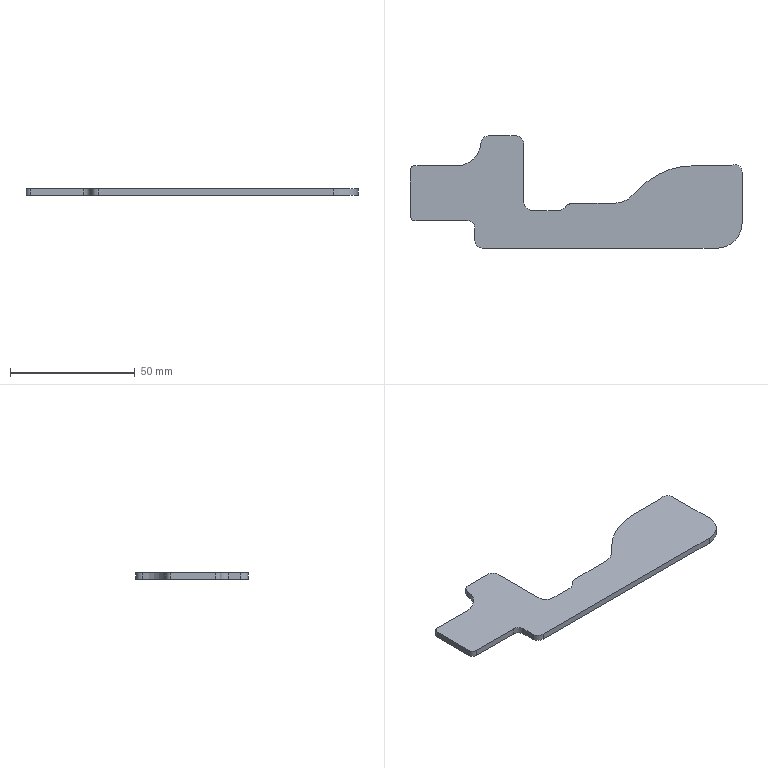Part | STEP file | lll_id334_x_t | 1 solid | 35 faces | box 133 x 45 x 2.5 mm | volume 8795 mm3 | cylinder 20 | plane 15 | commonest cylinder face diameters 6 x6 20 x3 4 x2 8 x2 6.716 x1 7.658 x1
STEP:
#1=CARTESIAN_POINT('',(1397.315,25.497,0.));
#2=VERTEX_POINT('',#1);
#3=CARTESIAN_POINT('',(1399.134,25.498,0.));
#4=VERTEX_POINT('',#3);
#5=CARTESIAN_POINT('',(1397.315,25.497,0.));
#6=DIRECTION('',(1.,0.0004734,0.));
#7=VECTOR('',#6,1.);
#8=LINE('',#5,#7);
#9=EDGE_CURVE('',#2,#4,#8,.T.);
#10=ORIENTED_EDGE('',*,*,#9,.F.);
#11=CARTESIAN_POINT('',(1397.315,25.497,2.5));
#12=VERTEX_POINT('',#11);
#13=CARTESIAN_POINT('',(1397.315,25.497,2.5));
#14=DIRECTION('',(0.,0.,-1.));
#15=VECTOR('',#14,1.);
#16=LINE('',#13,#15);
#17=EDGE_CURVE('',#12,#2,#16,.T.);
#18=ORIENTED_EDGE('',*,*,#17,.F.);
#19=CARTESIAN_POINT('',(1399.134,25.498,2.5));
#20=VERTEX_POINT('',#19);
#21=CARTESIAN_POINT('',(1397.315,25.497,2.5));
#22=DIRECTION('',(1.,0.0004734,0.));
#23=VECTOR('',#22,1.);
#24=LINE('',#21,#23);
#25=EDGE_CURVE('',#12,#20,#24,.T.);
#26=ORIENTED_EDGE('',*,*,#25,.T.);
#27=CARTESIAN_POINT('',(1399.134,25.498,2.5));
#28=DIRECTION('',(0.,0.,-1.));
#29=VECTOR('',#28,1.);
#30=LINE('',#27,#29);
#31=EDGE_CURVE('',#20,#4,#30,.T.);
#32=ORIENTED_EDGE('',*,*,#31,.T.);
#33=EDGE_LOOP('',(#10,#18,#26,#32));
#34=FACE_OUTER_BOUND('',#33,.T.);
#35=CARTESIAN_POINT('',(1397.315,25.497,2.5));
#36=DIRECTION('',(-0.0004734,1.,0.));
#37=DIRECTION('',(-1.,-0.0004734,0.));
#38=AXIS2_PLACEMENT_3D('',#35,#36,#37);
#39=PLANE('',#38);
#40=ADVANCED_FACE('',(#34),#39,.T.);
#41=CARTESIAN_POINT('',(1413.865,25.504,0.));
#42=VERTEX_POINT('',#41);
#43=CARTESIAN_POINT('',(1399.134,25.498,0.));
#44=DIRECTION('',(1.,0.0004015,0.));
#45=VECTOR('',#44,1.);
#46=LINE('',#43,#45);
#47=EDGE_CURVE('',#4,#42,#46,.T.);
#48=ORIENTED_EDGE('',*,*,#47,.F.);
#49=ORIENTED_EDGE('',*,*,#31,.F.);
#50=CARTESIAN_POINT('',(1413.865,25.504,2.5));
#51=VERTEX_POINT('',#50);
#52=CARTESIAN_POINT('',(1399.134,25.498,2.5));
#53=DIRECTION('',(1.,0.0004015,0.));
#54=VECTOR('',#53,1.);
#55=LINE('',#52,#54);
#56=EDGE_CURVE('',#20,#51,#55,.T.);
#57=ORIENTED_EDGE('',*,*,#56,.T.);
#58=CARTESIAN_POINT('',(1413.865,25.504,2.5));
#59=DIRECTION('',(0.,0.,-1.));
#60=VECTOR('',#59,1.);
#61=LINE('',#58,#60);
#62=EDGE_CURVE('',#51,#42,#61,.T.);
#63=ORIENTED_EDGE('',*,*,#62,.T.);
#64=EDGE_LOOP('',(#48,#49,#57,#63));
#65=FACE_OUTER_BOUND('',#64,.T.);
#66=CARTESIAN_POINT('',(1399.134,25.498,2.5));
#67=DIRECTION('',(-0.0004015,1.,0.));
#68=DIRECTION('',(-1.,-0.0004015,0.));
#69=AXIS2_PLACEMENT_3D('',#66,#67,#68);
#70=PLANE('',#69);
#71=ADVANCED_FACE('',(#65),#70,.T.);
#72=CARTESIAN_POINT('',(1420.933,28.433,0.));
#73=VERTEX_POINT('',#72);
#74=CARTESIAN_POINT('',(1413.861,35.504,0.));
#75=DIRECTION('',(0.,0.,1.));
#76=DIRECTION('',(1.,0.,0.));
#77=AXIS2_PLACEMENT_3D('',#74,#75,#76);
#78=CIRCLE('',#77,10.);
#79=EDGE_CURVE('',#42,#73,#78,.T.);
#80=ORIENTED_EDGE('',*,*,#79,.F.);
#81=ORIENTED_EDGE('',*,*,#62,.F.);
#82=CARTESIAN_POINT('',(1420.933,28.433,2.5));
#83=VERTEX_POINT('',#82);
#84=CARTESIAN_POINT('',(1413.861,35.504,2.5));
#85=DIRECTION('',(0.,0.,1.));
#86=DIRECTION('',(1.,0.,0.));
#87=AXIS2_PLACEMENT_3D('',#84,#85,#86);
#88=CIRCLE('',#87,10.);
#89=EDGE_CURVE('',#51,#83,#88,.T.);
#90=ORIENTED_EDGE('',*,*,#89,.T.);
#91=CARTESIAN_POINT('',(1420.933,28.433,2.5));
#92=DIRECTION('',(0.,0.,-1.));
#93=VECTOR('',#92,1.);
#94=LINE('',#91,#93);
#95=EDGE_CURVE('',#83,#73,#94,.T.);
#96=ORIENTED_EDGE('',*,*,#95,.T.);
#97=EDGE_LOOP('',(#80,#81,#90,#96));
#98=FACE_OUTER_BOUND('',#97,.T.);
#99=CARTESIAN_POINT('',(1413.861,35.504,2.5));
#100=DIRECTION('',(0.,0.,-1.));
#101=DIRECTION('',(-1.,0.,0.));
#102=AXIS2_PLACEMENT_3D('',#99,#100,#101);
#103=CYLINDRICAL_SURFACE('',#102,10.);
#104=ADVANCED_FACE('',(#98),#103,.F.);
#105=CARTESIAN_POINT('',(1424.213,31.713,0.));
#106=VERTEX_POINT('',#105);
#107=CARTESIAN_POINT('',(1420.933,28.433,0.));
#108=DIRECTION('',(0.7071,0.7071,0.));
#109=VECTOR('',#108,1.);
#110=LINE('',#107,#109);
#111=EDGE_CURVE('',#73,#106,#110,.T.);
#112=ORIENTED_EDGE('',*,*,#111,.F.);
#113=ORIENTED_EDGE('',*,*,#95,.F.);
#114=CARTESIAN_POINT('',(1424.213,31.713,2.5));
#115=VERTEX_POINT('',#114);
#116=CARTESIAN_POINT('',(1420.933,28.433,2.5));
#117=DIRECTION('',(0.7071,0.7071,0.));
#118=VECTOR('',#117,1.);
#119=LINE('',#116,#118);
#120=EDGE_CURVE('',#83,#115,#119,.T.);
#121=ORIENTED_EDGE('',*,*,#120,.T.);
#122=CARTESIAN_POINT('',(1424.213,31.713,2.5));
#123=DIRECTION('',(0.,0.,-1.));
#124=VECTOR('',#123,1.);
#125=LINE('',#122,#124);
#126=EDGE_CURVE('',#115,#106,#125,.T.);
#127=ORIENTED_EDGE('',*,*,#126,.T.);
#128=EDGE_LOOP('',(#112,#113,#121,#127));
#129=FACE_OUTER_BOUND('',#128,.T.);
#130=CARTESIAN_POINT('',(1420.933,28.433,2.5));
#131=DIRECTION('',(-0.7071,0.7071,0.));
#132=DIRECTION('',(-0.7071,-0.7071,0.));
#133=AXIS2_PLACEMENT_3D('',#130,#131,#132);
#134=PLANE('',#133);
#135=ADVANCED_FACE('',(#129),#134,.T.);
#136=CARTESIAN_POINT('',(1445.426,40.5,0.));
#137=VERTEX_POINT('',#136);
#138=CARTESIAN_POINT('',(1445.426,10.502,0.));
#139=DIRECTION('',(0.,0.,-1.));
#140=DIRECTION('',(1.,0.,0.));
#141=AXIS2_PLACEMENT_3D('',#138,#139,#140);
#142=CIRCLE('',#141,29.998);
#143=EDGE_CURVE('',#106,#137,#142,.T.);
#144=ORIENTED_EDGE('',*,*,#143,.F.);
#145=ORIENTED_EDGE('',*,*,#126,.F.);
#146=CARTESIAN_POINT('',(1445.426,40.5,2.5));
#147=VERTEX_POINT('',#146);
#148=CARTESIAN_POINT('',(1445.426,10.502,2.5));
#149=DIRECTION('',(0.,0.,-1.));
#150=DIRECTION('',(1.,0.,0.));
#151=AXIS2_PLACEMENT_3D('',#148,#149,#150);
#152=CIRCLE('',#151,29.998);
#153=EDGE_CURVE('',#115,#147,#152,.T.);
#154=ORIENTED_EDGE('',*,*,#153,.T.);
#155=CARTESIAN_POINT('',(1445.426,40.5,2.5));
#156=DIRECTION('',(0.,0.,-1.));
#157=VECTOR('',#156,1.);
#158=LINE('',#155,#157);
#159=EDGE_CURVE('',#147,#137,#158,.T.);
#160=ORIENTED_EDGE('',*,*,#159,.T.);
#161=EDGE_LOOP('',(#144,#145,#154,#160));
#162=FACE_OUTER_BOUND('',#161,.T.);
#163=CARTESIAN_POINT('',(1445.426,10.502,2.5));
#164=DIRECTION('',(0.,0.,-1.));
#165=DIRECTION('',(-1.,0.,0.));
#166=AXIS2_PLACEMENT_3D('',#163,#164,#165);
#167=CYLINDRICAL_SURFACE('',#166,29.998);
#168=ADVANCED_FACE('',(#162),#167,.T.);
#169=CARTESIAN_POINT('',(1459.602,40.5,0.));
#170=VERTEX_POINT('',#169);
#171=CARTESIAN_POINT('',(1445.426,40.5,0.));
#172=DIRECTION('',(1.,0.,0.));
#173=VECTOR('',#172,1.);
#174=LINE('',#171,#173);
#175=EDGE_CURVE('',#137,#170,#174,.T.);
#176=ORIENTED_EDGE('',*,*,#175,.F.);
#177=ORIENTED_EDGE('',*,*,#159,.F.);
#178=CARTESIAN_POINT('',(1459.602,40.5,2.5));
#179=VERTEX_POINT('',#178);
#180=CARTESIAN_POINT('',(1445.426,40.5,2.5));
#181=DIRECTION('',(1.,0.,0.));
#182=VECTOR('',#181,1.);
#183=LINE('',#180,#182);
#184=EDGE_CURVE('',#147,#179,#183,.T.);
#185=ORIENTED_EDGE('',*,*,#184,.T.);
#186=CARTESIAN_POINT('',(1459.602,40.5,2.5));
#187=DIRECTION('',(0.,0.,-1.));
#188=VECTOR('',#187,1.);
#189=LINE('',#186,#188);
#190=EDGE_CURVE('',#179,#170,#189,.T.);
#191=ORIENTED_EDGE('',*,*,#190,.T.);
#192=EDGE_LOOP('',(#176,#177,#185,#191));
#193=FACE_OUTER_BOUND('',#192,.T.);
#194=CARTESIAN_POINT('',(1445.426,40.5,2.5));
#195=DIRECTION('',(0.,1.,0.));
#196=DIRECTION('',(-1.,0.,0.));
#197=AXIS2_PLACEMENT_3D('',#194,#195,#196);
#198=PLANE('',#197);
#199=ADVANCED_FACE('',(#193),#198,.T.);
#200=CARTESIAN_POINT('',(1460.801,40.75,0.));
#201=VERTEX_POINT('',#200);
#202=CARTESIAN_POINT('',(1459.602,43.5,0.));
#203=DIRECTION('',(0.,0.,1.));
#204=DIRECTION('',(1.,0.,0.));
#205=AXIS2_PLACEMENT_3D('',#202,#203,#204);
#206=CIRCLE('',#205,3.);
#207=EDGE_CURVE('',#170,#201,#206,.T.);
#208=ORIENTED_EDGE('',*,*,#207,.F.);
#209=ORIENTED_EDGE('',*,*,#190,.F.);
#210=CARTESIAN_POINT('',(1460.801,40.75,2.5));
#211=VERTEX_POINT('',#210);
#212=CARTESIAN_POINT('',(1459.602,43.5,2.5));
#213=DIRECTION('',(0.,0.,1.));
#214=DIRECTION('',(1.,0.,0.));
#215=AXIS2_PLACEMENT_3D('',#212,#213,#214);
#216=CIRCLE('',#215,3.);
#217=EDGE_CURVE('',#179,#211,#216,.T.);
#218=ORIENTED_EDGE('',*,*,#217,.T.);
#219=CARTESIAN_POINT('',(1460.801,40.75,2.5));
#220=DIRECTION('',(0.,0.,-1.));
#221=VECTOR('',#220,1.);
#222=LINE('',#219,#221);
#223=EDGE_CURVE('',#211,#201,#222,.T.);
#224=ORIENTED_EDGE('',*,*,#223,.T.);
#225=EDGE_LOOP('',(#208,#209,#218,#224));
#226=FACE_OUTER_BOUND('',#225,.T.);
#227=CARTESIAN_POINT('',(1459.602,43.5,2.5));
#228=DIRECTION('',(0.,0.,-1.));
#229=DIRECTION('',(-1.,0.,0.));
#230=AXIS2_PLACEMENT_3D('',#227,#228,#229);
#231=CYLINDRICAL_SURFACE('',#230,3.);
#232=ADVANCED_FACE('',(#226),#231,.F.);
#233=CARTESIAN_POINT('',(1465.,38.,0.));
#234=VERTEX_POINT('',#233);
#235=CARTESIAN_POINT('',(1462.,38.,0.));
#236=DIRECTION('',(0.,0.,-1.));
#237=DIRECTION('',(1.,0.,0.));
#238=AXIS2_PLACEMENT_3D('',#235,#236,#237);
#239=CIRCLE('',#238,3.);
#240=EDGE_CURVE('',#201,#234,#239,.T.);
#241=ORIENTED_EDGE('',*,*,#240,.F.);
#242=ORIENTED_EDGE('',*,*,#223,.F.);
#243=CARTESIAN_POINT('',(1465.,38.,2.5));
#244=VERTEX_POINT('',#243);
#245=CARTESIAN_POINT('',(1462.,38.,2.5));
#246=DIRECTION('',(0.,0.,-1.));
#247=DIRECTION('',(1.,0.,0.));
#248=AXIS2_PLACEMENT_3D('',#245,#246,#247);
#249=CIRCLE('',#248,3.);
#250=EDGE_CURVE('',#211,#244,#249,.T.);
#251=ORIENTED_EDGE('',*,*,#250,.T.);
#252=CARTESIAN_POINT('',(1465.,38.,2.5));
#253=DIRECTION('',(0.,0.,-1.));
#254=VECTOR('',#253,1.);
#255=LINE('',#252,#254);
#256=EDGE_CURVE('',#244,#234,#255,.T.);
#257=ORIENTED_EDGE('',*,*,#256,.T.);
#258=EDGE_LOOP('',(#241,#242,#251,#257));
#259=FACE_OUTER_BOUND('',#258,.T.);
#260=CARTESIAN_POINT('',(1462.,38.,2.5));
#261=DIRECTION('',(0.,0.,-1.));
#262=DIRECTION('',(-1.,0.,0.));
#263=AXIS2_PLACEMENT_3D('',#260,#261,#262);
#264=CYLINDRICAL_SURFACE('',#263,3.);
#265=ADVANCED_FACE('',(#259),#264,.T.);
#266=CARTESIAN_POINT('',(1465.,17.5,0.));
#267=VERTEX_POINT('',#266);
#268=CARTESIAN_POINT('',(1465.,38.,0.));
#269=DIRECTION('',(0.,-1.,0.));
#270=VECTOR('',#269,1.);
#271=LINE('',#268,#270);
#272=EDGE_CURVE('',#234,#267,#271,.T.);
#273=ORIENTED_EDGE('',*,*,#272,.F.);
#274=ORIENTED_EDGE('',*,*,#256,.F.);
#275=CARTESIAN_POINT('',(1465.,17.5,2.5));
#276=VERTEX_POINT('',#275);
#277=CARTESIAN_POINT('',(1465.,38.,2.5));
#278=DIRECTION('',(0.,-1.,0.));
#279=VECTOR('',#278,1.);
#280=LINE('',#277,#279);
#281=EDGE_CURVE('',#244,#276,#280,.T.);
#282=ORIENTED_EDGE('',*,*,#281,.T.);
#283=CARTESIAN_POINT('',(1465.,17.5,2.5));
#284=DIRECTION('',(0.,0.,-1.));
#285=VECTOR('',#284,1.);
#286=LINE('',#283,#285);
#287=EDGE_CURVE('',#276,#267,#286,.T.);
#288=ORIENTED_EDGE('',*,*,#287,.T.);
#289=EDGE_LOOP('',(#273,#274,#282,#288));
#290=FACE_OUTER_BOUND('',#289,.T.);
#291=CARTESIAN_POINT('',(1465.,38.,2.5));
#292=DIRECTION('',(1.,0.,0.));
#293=DIRECTION('',(0.,0.,-1.));
#294=AXIS2_PLACEMENT_3D('',#291,#292,#293);
#295=PLANE('',#294);
#296=ADVANCED_FACE('',(#290),#295,.T.);
#297=CARTESIAN_POINT('',(1455.,7.5,0.));
#298=VERTEX_POINT('',#297);
#299=CARTESIAN_POINT('',(1455.,17.5,0.));
#300=DIRECTION('',(0.,0.,-1.));
#301=DIRECTION('',(1.,0.,0.));
#302=AXIS2_PLACEMENT_3D('',#299,#300,#301);
#303=CIRCLE('',#302,10.);
#304=EDGE_CURVE('',#267,#298,#303,.T.);
#305=ORIENTED_EDGE('',*,*,#304,.F.);
#306=ORIENTED_EDGE('',*,*,#287,.F.);
#307=CARTESIAN_POINT('',(1455.,7.5,2.5));
#308=VERTEX_POINT('',#307);
#309=CARTESIAN_POINT('',(1455.,17.5,2.5));
#310=DIRECTION('',(0.,0.,-1.));
#311=DIRECTION('',(1.,0.,0.));
#312=AXIS2_PLACEMENT_3D('',#309,#310,#311);
#313=CIRCLE('',#312,10.);
#314=EDGE_CURVE('',#276,#308,#313,.T.);
#315=ORIENTED_EDGE('',*,*,#314,.T.);
#316=CARTESIAN_POINT('',(1455.,7.5,2.5));
#317=DIRECTION('',(0.,0.,-1.));
#318=VECTOR('',#317,1.);
#319=LINE('',#316,#318);
#320=EDGE_CURVE('',#308,#298,#319,.T.);
#321=ORIENTED_EDGE('',*,*,#320,.T.);
#322=EDGE_LOOP('',(#305,#306,#315,#321));
#323=FACE_OUTER_BOUND('',#322,.T.);
#324=CARTESIAN_POINT('',(1455.,17.5,2.5));
#325=DIRECTION('',(0.,0.,-1.));
#326=DIRECTION('',(-1.,0.,0.));
#327=AXIS2_PLACEMENT_3D('',#324,#325,#326);
#328=CYLINDRICAL_SURFACE('',#327,10.);
#329=ADVANCED_FACE('',(#323),#328,.T.);
#330=CARTESIAN_POINT('',(1361.,7.5,0.));
#331=VERTEX_POINT('',#330);
#332=CARTESIAN_POINT('',(1455.,7.5,0.));
#333=DIRECTION('',(-1.,0.,0.));
#334=VECTOR('',#333,1.);
#335=LINE('',#332,#334);
#336=EDGE_CURVE('',#298,#331,#335,.T.);
#337=ORIENTED_EDGE('',*,*,#336,.F.);
#338=ORIENTED_EDGE('',*,*,#320,.F.);
#339=CARTESIAN_POINT('',(1361.,7.5,2.5));
#340=VERTEX_POINT('',#339);
#341=CARTESIAN_POINT('',(1455.,7.5,2.5));
#342=DIRECTION('',(-1.,0.,0.));
#343=VECTOR('',#342,1.);
#344=LINE('',#341,#343);
#345=EDGE_CURVE('',#308,#340,#344,.T.);
#346=ORIENTED_EDGE('',*,*,#345,.T.);
#347=CARTESIAN_POINT('',(1361.,7.5,2.5));
#348=DIRECTION('',(0.,0.,-1.));
#349=VECTOR('',#348,1.);
#350=LINE('',#347,#349);
#351=EDGE_CURVE('',#340,#331,#350,.T.);
#352=ORIENTED_EDGE('',*,*,#351,.T.);
#353=EDGE_LOOP('',(#337,#338,#346,#352));
#354=FACE_OUTER_BOUND('',#353,.T.);
#355=CARTESIAN_POINT('',(1455.,7.5,2.5));
#356=DIRECTION('',(0.,-1.,0.));
#357=DIRECTION('',(1.,0.,0.));
#358=AXIS2_PLACEMENT_3D('',#355,#356,#357);
#359=PLANE('',#358);
#360=ADVANCED_FACE('',(#354),#359,.T.);
#361=CARTESIAN_POINT('',(1358.,10.5,0.));
#362=VERTEX_POINT('',#361);
#363=CARTESIAN_POINT('',(1361.,10.5,0.));
#364=DIRECTION('',(0.,0.,-1.));
#365=DIRECTION('',(1.,0.,0.));
#366=AXIS2_PLACEMENT_3D('',#363,#364,#365);
#367=CIRCLE('',#366,3.);
#368=EDGE_CURVE('',#331,#362,#367,.T.);
#369=ORIENTED_EDGE('',*,*,#368,.F.);
#370=ORIENTED_EDGE('',*,*,#351,.F.);
#371=CARTESIAN_POINT('',(1358.,10.5,2.5));
#372=VERTEX_POINT('',#371);
#373=CARTESIAN_POINT('',(1361.,10.5,2.5));
#374=DIRECTION('',(0.,0.,-1.));
#375=DIRECTION('',(1.,0.,0.));
#376=AXIS2_PLACEMENT_3D('',#373,#374,#375);
#377=CIRCLE('',#376,3.);
#378=EDGE_CURVE('',#340,#372,#377,.T.);
#379=ORIENTED_EDGE('',*,*,#378,.T.);
#380=CARTESIAN_POINT('',(1358.,10.5,2.5));
#381=DIRECTION('',(0.,0.,-1.));
#382=VECTOR('',#381,1.);
#383=LINE('',#380,#382);
#384=EDGE_CURVE('',#372,#362,#383,.T.);
#385=ORIENTED_EDGE('',*,*,#384,.T.);
#386=EDGE_LOOP('',(#369,#370,#379,#385));
#387=FACE_OUTER_BOUND('',#386,.T.);
#388=CARTESIAN_POINT('',(1361.,10.5,2.5));
#389=DIRECTION('',(0.,0.,-1.));
#390=DIRECTION('',(-1.,0.,0.));
#391=AXIS2_PLACEMENT_3D('',#388,#389,#390);
#392=CYLINDRICAL_SURFACE('',#391,3.);
#393=ADVANCED_FACE('',(#387),#392,.T.);
#394=CARTESIAN_POINT('',(1358.,15.5,0.));
#395=VERTEX_POINT('',#394);
#396=CARTESIAN_POINT('',(1358.,10.5,0.));
#397=DIRECTION('',(0.,1.,0.));
#398=VECTOR('',#397,1.);
#399=LINE('',#396,#398);
#400=EDGE_CURVE('',#362,#395,#399,.T.);
#401=ORIENTED_EDGE('',*,*,#400,.F.);
#402=ORIENTED_EDGE('',*,*,#384,.F.);
#403=CARTESIAN_POINT('',(1358.,15.5,2.5));
#404=VERTEX_POINT('',#403);
#405=CARTESIAN_POINT('',(1358.,10.5,2.5));
#406=DIRECTION('',(0.,1.,0.));
#407=VECTOR('',#406,1.);
#408=LINE('',#405,#407);
#409=EDGE_CURVE('',#372,#404,#408,.T.);
#410=ORIENTED_EDGE('',*,*,#409,.T.);
#411=CARTESIAN_POINT('',(1358.,15.5,2.5));
#412=DIRECTION('',(0.,0.,-1.));
#413=VECTOR('',#412,1.);
#414=LINE('',#411,#413);
#415=EDGE_CURVE('',#404,#395,#414,.T.);
#416=ORIENTED_EDGE('',*,*,#415,.T.);
#417=EDGE_LOOP('',(#401,#402,#410,#416));
#418=FACE_OUTER_BOUND('',#417,.T.);
#419=CARTESIAN_POINT('',(1358.,10.5,2.5));
#420=DIRECTION('',(-1.,0.,0.));
#421=DIRECTION('',(0.,-1.,0.));
#422=AXIS2_PLACEMENT_3D('',#419,#420,#421);
#423=PLANE('',#422);
#424=ADVANCED_FACE('',(#418),#423,.T.);
#425=CARTESIAN_POINT('',(1355.,18.5,0.));
#426=VERTEX_POINT('',#425);
#427=CARTESIAN_POINT('',(1355.,15.5,0.));
#428=DIRECTION('',(0.,0.,1.));
#429=DIRECTION('',(1.,0.,0.));
#430=AXIS2_PLACEMENT_3D('',#427,#428,#429);
#431=CIRCLE('',#430,3.);
#432=EDGE_CURVE('',#395,#426,#431,.T.);
#433=ORIENTED_EDGE('',*,*,#432,.F.);
#434=ORIENTED_EDGE('',*,*,#415,.F.);
#435=CARTESIAN_POINT('',(1355.,18.5,2.5));
#436=VERTEX_POINT('',#435);
#437=CARTESIAN_POINT('',(1355.,15.5,2.5));
#438=DIRECTION('',(0.,0.,1.));
#439=DIRECTION('',(1.,0.,0.));
#440=AXIS2_PLACEMENT_3D('',#437,#438,#439);
#441=CIRCLE('',#440,3.);
#442=EDGE_CURVE('',#404,#436,#441,.T.);
#443=ORIENTED_EDGE('',*,*,#442,.T.);
#444=CARTESIAN_POINT('',(1355.,18.5,2.5));
#445=DIRECTION('',(0.,0.,-1.));
#446=VECTOR('',#445,1.);
#447=LINE('',#444,#446);
#448=EDGE_CURVE('',#436,#426,#447,.T.);
#449=ORIENTED_EDGE('',*,*,#448,.T.);
#450=EDGE_LOOP('',(#433,#434,#443,#449));
#451=FACE_OUTER_BOUND('',#450,.T.);
#452=CARTESIAN_POINT('',(1355.,15.5,2.5));
#453=DIRECTION('',(0.,0.,-1.));
#454=DIRECTION('',(-1.,0.,0.));
#455=AXIS2_PLACEMENT_3D('',#452,#453,#454);
#456=CYLINDRICAL_SURFACE('',#455,3.);
#457=ADVANCED_FACE('',(#451),#456,.F.);
#458=CARTESIAN_POINT('',(1334.,18.5,0.));
#459=VERTEX_POINT('',#458);
#460=CARTESIAN_POINT('',(1355.,18.5,0.));
#461=DIRECTION('',(-1.,0.,0.));
#462=VECTOR('',#461,1.);
#463=LINE('',#460,#462);
#464=EDGE_CURVE('',#426,#459,#463,.T.);
#465=ORIENTED_EDGE('',*,*,#464,.F.);
#466=ORIENTED_EDGE('',*,*,#448,.F.);
#467=CARTESIAN_POINT('',(1334.,18.5,2.5));
#468=VERTEX_POINT('',#467);
#469=CARTESIAN_POINT('',(1355.,18.5,2.5));
#470=DIRECTION('',(-1.,0.,0.));
#471=VECTOR('',#470,1.);
#472=LINE('',#469,#471);
#473=EDGE_CURVE('',#436,#468,#472,.T.);
#474=ORIENTED_EDGE('',*,*,#473,.T.);
#475=CARTESIAN_POINT('',(1334.,18.5,2.5));
#476=DIRECTION('',(0.,0.,-1.));
#477=VECTOR('',#476,1.);
#478=LINE('',#475,#477);
#479=EDGE_CURVE('',#468,#459,#478,.T.);
#480=ORIENTED_EDGE('',*,*,#479,.T.);
#481=EDGE_LOOP('',(#465,#466,#474,#480));
#482=FACE_OUTER_BOUND('',#481,.T.);
#483=CARTESIAN_POINT('',(1355.,18.5,2.5));
#484=DIRECTION('',(0.,-1.,0.));
#485=DIRECTION('',(1.,0.,0.));
#486=AXIS2_PLACEMENT_3D('',#483,#484,#485);
#487=PLANE('',#486);
#488=ADVANCED_FACE('',(#482),#487,.T.);
#489=CARTESIAN_POINT('',(1332.,20.5,0.));
#490=VERTEX_POINT('',#489);
#491=CARTESIAN_POINT('',(1334.,20.5,0.));
#492=DIRECTION('',(0.,0.,-1.));
#493=DIRECTION('',(1.,0.,0.));
#494=AXIS2_PLACEMENT_3D('',#491,#492,#493);
#495=CIRCLE('',#494,2.);
#496=EDGE_CURVE('',#459,#490,#495,.T.);
#497=ORIENTED_EDGE('',*,*,#496,.F.);
#498=ORIENTED_EDGE('',*,*,#479,.F.);
#499=CARTESIAN_POINT('',(1332.,20.5,2.5));
#500=VERTEX_POINT('',#499);
#501=CARTESIAN_POINT('',(1334.,20.5,2.5));
#502=DIRECTION('',(0.,0.,-1.));
#503=DIRECTION('',(1.,0.,0.));
#504=AXIS2_PLACEMENT_3D('',#501,#502,#503);
#505=CIRCLE('',#504,2.);
#506=EDGE_CURVE('',#468,#500,#505,.T.);
#507=ORIENTED_EDGE('',*,*,#506,.T.);
#508=CARTESIAN_POINT('',(1332.,20.5,2.5));
#509=DIRECTION('',(0.,0.,-1.));
#510=VECTOR('',#509,1.);
#511=LINE('',#508,#510);
#512=EDGE_CURVE('',#500,#490,#511,.T.);
#513=ORIENTED_EDGE('',*,*,#512,.T.);
#514=EDGE_LOOP('',(#497,#498,#507,#513));
#515=FACE_OUTER_BOUND('',#514,.T.);
#516=CARTESIAN_POINT('',(1334.,20.5,2.5));
#517=DIRECTION('',(0.,0.,-1.));
#518=DIRECTION('',(-1.,0.,0.));
#519=AXIS2_PLACEMENT_3D('',#516,#517,#518);
#520=CYLINDRICAL_SURFACE('',#519,2.);
#521=ADVANCED_FACE('',(#515),#520,.T.);
#522=CARTESIAN_POINT('',(1332.,38.5,0.));
#523=VERTEX_POINT('',#522);
#524=CARTESIAN_POINT('',(1332.,20.5,0.));
#525=DIRECTION('',(0.,1.,0.));
#526=VECTOR('',#525,1.);
#527=LINE('',#524,#526);
#528=EDGE_CURVE('',#490,#523,#527,.T.);
#529=ORIENTED_EDGE('',*,*,#528,.F.);
#530=ORIENTED_EDGE('',*,*,#512,.F.);
#531=CARTESIAN_POINT('',(1332.,38.5,2.5));
#532=VERTEX_POINT('',#531);
#533=CARTESIAN_POINT('',(1332.,20.5,2.5));
#534=DIRECTION('',(0.,1.,0.));
#535=VECTOR('',#534,1.);
#536=LINE('',#533,#535);
#537=EDGE_CURVE('',#500,#532,#536,.T.);
#538=ORIENTED_EDGE('',*,*,#537,.T.);
#539=CARTESIAN_POINT('',(1332.,38.5,2.5));
#540=DIRECTION('',(0.,0.,-1.));
#541=VECTOR('',#540,1.);
#542=LINE('',#539,#541);
#543=EDGE_CURVE('',#532,#523,#542,.T.);
#544=ORIENTED_EDGE('',*,*,#543,.T.);
#545=EDGE_LOOP('',(#529,#530,#538,#544));
#546=FACE_OUTER_BOUND('',#545,.T.);
#547=CARTESIAN_POINT('',(1332.,20.5,2.5));
#548=DIRECTION('',(-1.,0.,0.));
#549=DIRECTION('',(0.,0.,1.));
#550=AXIS2_PLACEMENT_3D('',#547,#548,#549);
#551=PLANE('',#550);
#552=ADVANCED_FACE('',(#546),#551,.T.);
#553=CARTESIAN_POINT('',(1334.,40.5,0.));
#554=VERTEX_POINT('',#553);
#555=CARTESIAN_POINT('',(1334.,38.5,0.));
#556=DIRECTION('',(0.,0.,-1.));
#557=DIRECTION('',(1.,0.,0.));
#558=AXIS2_PLACEMENT_3D('',#555,#556,#557);
#559=CIRCLE('',#558,2.);
#560=EDGE_CURVE('',#523,#554,#559,.T.);
#561=ORIENTED_EDGE('',*,*,#560,.F.);
#562=ORIENTED_EDGE('',*,*,#543,.F.);
#563=CARTESIAN_POINT('',(1334.,40.5,2.5));
#564=VERTEX_POINT('',#563);
#565=CARTESIAN_POINT('',(1334.,38.5,2.5));
#566=DIRECTION('',(0.,0.,-1.));
#567=DIRECTION('',(1.,0.,0.));
#568=AXIS2_PLACEMENT_3D('',#565,#566,#567);
#569=CIRCLE('',#568,2.);
#570=EDGE_CURVE('',#532,#564,#569,.T.);
#571=ORIENTED_EDGE('',*,*,#570,.T.);
#572=CARTESIAN_POINT('',(1334.,40.5,2.5));
#573=DIRECTION('',(0.,0.,-1.));
#574=VECTOR('',#573,1.);
#575=LINE('',#572,#574);
#576=EDGE_CURVE('',#564,#554,#575,.T.);
#577=ORIENTED_EDGE('',*,*,#576,.T.);
#578=EDGE_LOOP('',(#561,#562,#571,#577));
#579=FACE_OUTER_BOUND('',#578,.T.);
#580=CARTESIAN_POINT('',(1334.,38.5,2.5));
#581=DIRECTION('',(0.,0.,-1.));
#582=DIRECTION('',(-1.,0.,0.));
#583=AXIS2_PLACEMENT_3D('',#580,#581,#582);
#584=CYLINDRICAL_SURFACE('',#583,2.);
#585=ADVANCED_FACE('',(#579),#584,.T.);
#586=CARTESIAN_POINT('',(1350.5,40.5,0.));
#587=VERTEX_POINT('',#586);
#588=CARTESIAN_POINT('',(1334.,40.5,0.));
#589=DIRECTION('',(1.,0.,0.));
#590=VECTOR('',#589,1.);
#591=LINE('',#588,#590);
#592=EDGE_CURVE('',#554,#587,#591,.T.);
#593=ORIENTED_EDGE('',*,*,#592,.F.);
#594=ORIENTED_EDGE('',*,*,#576,.F.);
#595=CARTESIAN_POINT('',(1350.5,40.5,2.5));
#596=VERTEX_POINT('',#595);
#597=CARTESIAN_POINT('',(1334.,40.5,2.5));
#598=DIRECTION('',(1.,0.,0.));
#599=VECTOR('',#598,1.);
#600=LINE('',#597,#599);
#601=EDGE_CURVE('',#564,#596,#600,.T.);
#602=ORIENTED_EDGE('',*,*,#601,.T.);
#603=CARTESIAN_POINT('',(1350.5,40.5,2.5));
#604=DIRECTION('',(0.,0.,-1.));
#605=VECTOR('',#604,1.);
#606=LINE('',#603,#605);
#607=EDGE_CURVE('',#596,#587,#606,.T.);
#608=ORIENTED_EDGE('',*,*,#607,.T.);
#609=EDGE_LOOP('',(#593,#594,#602,#608));
#610=FACE_OUTER_BOUND('',#609,.T.);
#611=CARTESIAN_POINT('',(1334.,40.5,2.5));
#612=DIRECTION('',(0.,1.,0.));
#613=DIRECTION('',(-1.,0.,0.));
#614=AXIS2_PLACEMENT_3D('',#611,#612,#613);
#615=PLANE('',#614);
#616=ADVANCED_FACE('',(#610),#615,.T.);
#617=CARTESIAN_POINT('',(1360.47,49.731,0.));
#618=VERTEX_POINT('',#617);
#619=CARTESIAN_POINT('',(1350.5,50.5,0.));
#620=DIRECTION('',(0.,0.,1.));
#621=DIRECTION('',(1.,0.,0.));
#622=AXIS2_PLACEMENT_3D('',#619,#620,#621);
#623=CIRCLE('',#622,10.);
#624=EDGE_CURVE('',#587,#618,#623,.T.);
#625=ORIENTED_EDGE('',*,*,#624,.F.);
#626=ORIENTED_EDGE('',*,*,#607,.F.);
#627=CARTESIAN_POINT('',(1360.47,49.731,2.5));
#628=VERTEX_POINT('',#627);
#629=CARTESIAN_POINT('',(1350.5,50.5,2.5));
#630=DIRECTION('',(0.,0.,1.));
#631=DIRECTION('',(1.,0.,0.));
#632=AXIS2_PLACEMENT_3D('',#629,#630,#631);
#633=CIRCLE('',#632,10.);
#634=EDGE_CURVE('',#596,#628,#633,.T.);
#635=ORIENTED_EDGE('',*,*,#634,.T.);
#636=CARTESIAN_POINT('',(1360.47,49.731,2.5));
#637=DIRECTION('',(0.,0.,-1.));
#638=VECTOR('',#637,1.);
#639=LINE('',#636,#638);
#640=EDGE_CURVE('',#628,#618,#639,.T.);
#641=ORIENTED_EDGE('',*,*,#640,.T.);
#642=EDGE_LOOP('',(#625,#626,#635,#641));
#643=FACE_OUTER_BOUND('',#642,.T.);
#644=CARTESIAN_POINT('',(1350.5,50.5,2.5));
#645=DIRECTION('',(0.,0.,-1.));
#646=DIRECTION('',(-1.,0.,0.));
#647=AXIS2_PLACEMENT_3D('',#644,#645,#646);
#648=CYLINDRICAL_SURFACE('',#647,10.);
#649=ADVANCED_FACE('',(#643),#648,.F.);
#650=CARTESIAN_POINT('',(1363.461,52.5,0.));
#651=VERTEX_POINT('',#650);
#652=CARTESIAN_POINT('',(1363.461,49.5,0.));
#653=DIRECTION('',(0.,0.,-1.));
#654=DIRECTION('',(1.,0.,0.));
#655=AXIS2_PLACEMENT_3D('',#652,#653,#654);
#656=CIRCLE('',#655,3.);
#657=EDGE_CURVE('',#618,#651,#656,.T.);
#658=ORIENTED_EDGE('',*,*,#657,.F.);
#659=ORIENTED_EDGE('',*,*,#640,.F.);
#660=CARTESIAN_POINT('',(1363.461,52.5,2.5));
#661=VERTEX_POINT('',#660);
#662=CARTESIAN_POINT('',(1363.461,49.5,2.5));
#663=DIRECTION('',(0.,0.,-1.));
#664=DIRECTION('',(1.,0.,0.));
#665=AXIS2_PLACEMENT_3D('',#662,#663,#664);
#666=CIRCLE('',#665,3.);
#667=EDGE_CURVE('',#628,#661,#666,.T.);
#668=ORIENTED_EDGE('',*,*,#667,.T.);
#669=CARTESIAN_POINT('',(1363.461,52.5,2.5));
#670=DIRECTION('',(0.,0.,-1.));
#671=VECTOR('',#670,1.);
#672=LINE('',#669,#671);
#673=EDGE_CURVE('',#661,#651,#672,.T.);
#674=ORIENTED_EDGE('',*,*,#673,.T.);
#675=EDGE_LOOP('',(#658,#659,#668,#674));
#676=FACE_OUTER_BOUND('',#675,.T.);
#677=CARTESIAN_POINT('',(1363.461,49.5,2.5));
#678=DIRECTION('',(0.,0.,-1.));
#679=DIRECTION('',(-1.,0.,0.));
#680=AXIS2_PLACEMENT_3D('',#677,#678,#679);
#681=CYLINDRICAL_SURFACE('',#680,3.);
#682=ADVANCED_FACE('',(#676),#681,.T.);
#683=CARTESIAN_POINT('',(1374.507,52.5,0.));
#684=VERTEX_POINT('',#683);
#685=CARTESIAN_POINT('',(1363.461,52.5,0.));
#686=DIRECTION('',(1.,0.,0.));
#687=VECTOR('',#686,1.);
#688=LINE('',#685,#687);
#689=EDGE_CURVE('',#651,#684,#688,.T.);
#690=ORIENTED_EDGE('',*,*,#689,.F.);
#691=ORIENTED_EDGE('',*,*,#673,.F.);
#692=CARTESIAN_POINT('',(1374.507,52.5,2.5));
#693=VERTEX_POINT('',#692);
#694=CARTESIAN_POINT('',(1363.461,52.5,2.5));
#695=DIRECTION('',(1.,0.,0.));
#696=VECTOR('',#695,1.);
#697=LINE('',#694,#696);
#698=EDGE_CURVE('',#661,#693,#697,.T.);
#699=ORIENTED_EDGE('',*,*,#698,.T.);
#700=CARTESIAN_POINT('',(1374.507,52.5,2.5));
#701=DIRECTION('',(0.,0.,-1.));
#702=VECTOR('',#701,1.);
#703=LINE('',#700,#702);
#704=EDGE_CURVE('',#693,#684,#703,.T.);
#705=ORIENTED_EDGE('',*,*,#704,.T.);
#706=EDGE_LOOP('',(#690,#691,#699,#705));
#707=FACE_OUTER_BOUND('',#706,.T.);
#708=CARTESIAN_POINT('',(1363.461,52.5,2.5));
#709=DIRECTION('',(0.,1.,0.));
#710=DIRECTION('',(-1.,0.,0.));
#711=AXIS2_PLACEMENT_3D('',#708,#709,#710);
#712=PLANE('',#711);
#713=ADVANCED_FACE('',(#707),#712,.T.);
#714=CARTESIAN_POINT('',(1377.507,49.5,0.));
#715=VERTEX_POINT('',#714);
#716=CARTESIAN_POINT('',(1374.507,49.5,0.));
#717=DIRECTION('',(0.,0.,-1.));
#718=DIRECTION('',(1.,0.,0.));
#719=AXIS2_PLACEMENT_3D('',#716,#717,#718);
#720=CIRCLE('',#719,3.);
#721=EDGE_CURVE('',#684,#715,#720,.T.);
#722=ORIENTED_EDGE('',*,*,#721,.F.);
#723=ORIENTED_EDGE('',*,*,#704,.F.);
#724=CARTESIAN_POINT('',(1377.507,49.5,2.5));
#725=VERTEX_POINT('',#724);
#726=CARTESIAN_POINT('',(1374.507,49.5,2.5));
#727=DIRECTION('',(0.,0.,-1.));
#728=DIRECTION('',(1.,0.,0.));
#729=AXIS2_PLACEMENT_3D('',#726,#727,#728);
#730=CIRCLE('',#729,3.);
#731=EDGE_CURVE('',#693,#725,#730,.T.);
#732=ORIENTED_EDGE('',*,*,#731,.T.);
#733=CARTESIAN_POINT('',(1377.507,49.5,2.5));
#734=DIRECTION('',(0.,0.,-1.));
#735=VECTOR('',#734,1.);
#736=LINE('',#733,#735);
#737=EDGE_CURVE('',#725,#715,#736,.T.);
#738=ORIENTED_EDGE('',*,*,#737,.T.);
#739=EDGE_LOOP('',(#722,#723,#732,#738));
#740=FACE_OUTER_BOUND('',#739,.T.);
#741=CARTESIAN_POINT('',(1374.507,49.5,2.5));
#742=DIRECTION('',(0.,0.,-1.));
#743=DIRECTION('',(-1.,0.,0.));
#744=AXIS2_PLACEMENT_3D('',#741,#742,#743);
#745=CYLINDRICAL_SURFACE('',#744,3.);
#746=ADVANCED_FACE('',(#740),#745,.T.);
#747=CARTESIAN_POINT('',(1377.509,26.493,0.));
#748=VERTEX_POINT('',#747);
#749=CARTESIAN_POINT('',(1377.507,49.5,0.));
#750=DIRECTION('',(0.00008306,-1.,0.));
#751=VECTOR('',#750,1.);
#752=LINE('',#749,#751);
#753=EDGE_CURVE('',#715,#748,#752,.T.);
#754=ORIENTED_EDGE('',*,*,#753,.F.);
#755=ORIENTED_EDGE('',*,*,#737,.F.);
#756=CARTESIAN_POINT('',(1377.509,26.493,2.5));
#757=VERTEX_POINT('',#756);
#758=CARTESIAN_POINT('',(1377.507,49.5,2.5));
#759=DIRECTION('',(0.00008306,-1.,0.));
#760=VECTOR('',#759,1.);
#761=LINE('',#758,#760);
#762=EDGE_CURVE('',#725,#757,#761,.T.);
#763=ORIENTED_EDGE('',*,*,#762,.T.);
#764=CARTESIAN_POINT('',(1377.509,26.493,2.5));
#765=DIRECTION('',(0.,0.,-1.));
#766=VECTOR('',#765,1.);
#767=LINE('',#764,#766);
#768=EDGE_CURVE('',#757,#748,#767,.T.);
#769=ORIENTED_EDGE('',*,*,#768,.T.);
#770=EDGE_LOOP('',(#754,#755,#763,#769));
#771=FACE_OUTER_BOUND('',#770,.T.);
#772=CARTESIAN_POINT('',(1377.507,49.5,2.5));
#773=DIRECTION('',(1.,0.00008306,0.));
#774=DIRECTION('',(-0.00008306,1.,0.));
#775=AXIS2_PLACEMENT_3D('',#772,#773,#774);
#776=PLANE('',#775);
#777=ADVANCED_FACE('',(#771),#776,.T.);
#778=CARTESIAN_POINT('',(1381.51,22.493,0.));
#779=VERTEX_POINT('',#778);
#780=CARTESIAN_POINT('',(1381.509,26.493,0.));
#781=DIRECTION('',(0.,0.,1.));
#782=DIRECTION('',(1.,0.,0.));
#783=AXIS2_PLACEMENT_3D('',#780,#781,#782);
#784=CIRCLE('',#783,4.);
#785=EDGE_CURVE('',#748,#779,#784,.T.);
#786=ORIENTED_EDGE('',*,*,#785,.F.);
#787=ORIENTED_EDGE('',*,*,#768,.F.);
#788=CARTESIAN_POINT('',(1381.51,22.493,2.5));
#789=VERTEX_POINT('',#788);
#790=CARTESIAN_POINT('',(1381.509,26.493,2.5));
#791=DIRECTION('',(0.,0.,1.));
#792=DIRECTION('',(1.,0.,0.));
#793=AXIS2_PLACEMENT_3D('',#790,#791,#792);
#794=CIRCLE('',#793,4.);
#795=EDGE_CURVE('',#757,#789,#794,.T.);
#796=ORIENTED_EDGE('',*,*,#795,.T.);
#797=CARTESIAN_POINT('',(1381.51,22.493,2.5));
#798=DIRECTION('',(0.,0.,-1.));
#799=VECTOR('',#798,1.);
#800=LINE('',#797,#799);
#801=EDGE_CURVE('',#789,#779,#800,.T.);
#802=ORIENTED_EDGE('',*,*,#801,.T.);
#803=EDGE_LOOP('',(#786,#787,#796,#802));
#804=FACE_OUTER_BOUND('',#803,.T.);
#805=CARTESIAN_POINT('',(1381.509,26.493,2.5));
#806=DIRECTION('',(0.,0.,-1.));
#807=DIRECTION('',(-1.,0.,0.));
#808=AXIS2_PLACEMENT_3D('',#805,#806,#807);
#809=CYLINDRICAL_SURFACE('',#808,4.);
#810=ADVANCED_FACE('',(#804),#809,.F.);
#811=CARTESIAN_POINT('',(1391.,22.495,0.));
#812=VERTEX_POINT('',#811);
#813=CARTESIAN_POINT('',(1381.51,22.493,0.));
#814=DIRECTION('',(1.,0.0002273,0.));
#815=VECTOR('',#814,1.);
#816=LINE('',#813,#815);
#817=EDGE_CURVE('',#779,#812,#816,.T.);
#818=ORIENTED_EDGE('',*,*,#817,.F.);
#819=ORIENTED_EDGE('',*,*,#801,.F.);
#820=CARTESIAN_POINT('',(1391.,22.495,2.5));
#821=VERTEX_POINT('',#820);
#822=CARTESIAN_POINT('',(1381.51,22.493,2.5));
#823=DIRECTION('',(1.,0.0002273,0.));
#824=VECTOR('',#823,1.);
#825=LINE('',#822,#824);
#826=EDGE_CURVE('',#789,#821,#825,.T.);
#827=ORIENTED_EDGE('',*,*,#826,.T.);
#828=CARTESIAN_POINT('',(1391.,22.495,2.5));
#829=DIRECTION('',(0.,0.,-1.));
#830=VECTOR('',#829,1.);
#831=LINE('',#828,#830);
#832=EDGE_CURVE('',#821,#812,#831,.T.);
#833=ORIENTED_EDGE('',*,*,#832,.T.);
#834=EDGE_LOOP('',(#818,#819,#827,#833));
#835=FACE_OUTER_BOUND('',#834,.T.);
#836=CARTESIAN_POINT('',(1381.51,22.493,2.5));
#837=DIRECTION('',(-0.0002273,1.,0.));
#838=DIRECTION('',(-1.,-0.0002273,0.));
#839=AXIS2_PLACEMENT_3D('',#836,#837,#838);
#840=PLANE('',#839);
#841=ADVANCED_FACE('',(#835),#840,.T.);
#842=CARTESIAN_POINT('',(1394.112,23.983,0.));
#843=VERTEX_POINT('',#842);
#844=CARTESIAN_POINT('',(1390.999,26.495,0.));
#845=DIRECTION('',(0.,0.,1.));
#846=DIRECTION('',(1.,0.,0.));
#847=AXIS2_PLACEMENT_3D('',#844,#845,#846);
#848=CIRCLE('',#847,4.);
#849=EDGE_CURVE('',#812,#843,#848,.T.);
#850=ORIENTED_EDGE('',*,*,#849,.F.);
#851=ORIENTED_EDGE('',*,*,#832,.F.);
#852=CARTESIAN_POINT('',(1394.112,23.983,2.5));
#853=VERTEX_POINT('',#852);
#854=CARTESIAN_POINT('',(1390.999,26.495,2.5));
#855=DIRECTION('',(0.,0.,1.));
#856=DIRECTION('',(1.,0.,0.));
#857=AXIS2_PLACEMENT_3D('',#854,#855,#856);
#858=CIRCLE('',#857,4.);
#859=EDGE_CURVE('',#821,#853,#858,.T.);
#860=ORIENTED_EDGE('',*,*,#859,.T.);
#861=CARTESIAN_POINT('',(1394.112,23.983,2.5));
#862=DIRECTION('',(0.,0.,-1.));
#863=VECTOR('',#862,1.);
#864=LINE('',#861,#863);
#865=EDGE_CURVE('',#853,#843,#864,.T.);
#866=ORIENTED_EDGE('',*,*,#865,.T.);
#867=EDGE_LOOP('',(#850,#851,#860,#866));
#868=FACE_OUTER_BOUND('',#867,.T.);
#869=CARTESIAN_POINT('',(1390.999,26.495,2.5));
#870=DIRECTION('',(0.,0.,-1.));
#871=DIRECTION('',(-1.,0.,0.));
#872=AXIS2_PLACEMENT_3D('',#869,#870,#871);
#873=CYLINDRICAL_SURFACE('',#872,4.);
#874=ADVANCED_FACE('',(#868),#873,.F.);
#875=CARTESIAN_POINT('',(1394.775,24.627,0.));
#876=VERTEX_POINT('',#875);
#877=CARTESIAN_POINT('',(1397.092,21.579,0.));
#878=DIRECTION('',(0.,0.,-1.));
#879=DIRECTION('',(1.,0.,0.));
#880=AXIS2_PLACEMENT_3D('',#877,#878,#879);
#881=CIRCLE('',#880,3.829);
#882=EDGE_CURVE('',#843,#876,#881,.T.);
#883=ORIENTED_EDGE('',*,*,#882,.F.);
#884=ORIENTED_EDGE('',*,*,#865,.F.);
#885=CARTESIAN_POINT('',(1394.775,24.627,2.5));
#886=VERTEX_POINT('',#885);
#887=CARTESIAN_POINT('',(1397.092,21.579,2.5));
#888=DIRECTION('',(0.,0.,-1.));
#889=DIRECTION('',(1.,0.,0.));
#890=AXIS2_PLACEMENT_3D('',#887,#888,#889);
#891=CIRCLE('',#890,3.829);
#892=EDGE_CURVE('',#853,#886,#891,.T.);
#893=ORIENTED_EDGE('',*,*,#892,.T.);
#894=CARTESIAN_POINT('',(1394.775,24.627,2.5));
#895=DIRECTION('',(0.,0.,-1.));
#896=VECTOR('',#895,1.);
#897=LINE('',#894,#896);
#898=EDGE_CURVE('',#886,#876,#897,.T.);
#899=ORIENTED_EDGE('',*,*,#898,.T.);
#900=EDGE_LOOP('',(#883,#884,#893,#899));
#901=FACE_OUTER_BOUND('',#900,.T.);
#902=CARTESIAN_POINT('',(1397.092,21.579,2.5));
#903=DIRECTION('',(0.,0.,-1.));
#904=DIRECTION('',(-1.,0.,0.));
#905=AXIS2_PLACEMENT_3D('',#902,#903,#904);
#906=CYLINDRICAL_SURFACE('',#905,3.829);
#907=ADVANCED_FACE('',(#901),#906,.T.);
#908=CARTESIAN_POINT('',(1395.716,25.182,0.));
#909=VERTEX_POINT('',#908);
#910=CARTESIAN_POINT('',(1397.363,21.312,0.));
#911=DIRECTION('',(0.,0.,-1.));
#912=DIRECTION('',(1.,0.,0.));
#913=AXIS2_PLACEMENT_3D('',#910,#911,#912);
#914=CIRCLE('',#913,4.206);
#915=EDGE_CURVE('',#876,#909,#914,.T.);
#916=ORIENTED_EDGE('',*,*,#915,.F.);
#917=ORIENTED_EDGE('',*,*,#898,.F.);
#918=CARTESIAN_POINT('',(1395.716,25.182,2.5));
#919=VERTEX_POINT('',#918);
#920=CARTESIAN_POINT('',(1397.363,21.312,2.5));
#921=DIRECTION('',(0.,0.,-1.));
#922=DIRECTION('',(1.,0.,0.));
#923=AXIS2_PLACEMENT_3D('',#920,#921,#922);
#924=CIRCLE('',#923,4.206);
#925=EDGE_CURVE('',#886,#919,#924,.T.);
#926=ORIENTED_EDGE('',*,*,#925,.T.);
#927=CARTESIAN_POINT('',(1395.716,25.182,2.5));
#928=DIRECTION('',(0.,0.,-1.));
#929=VECTOR('',#928,1.);
#930=LINE('',#927,#929);
#931=EDGE_CURVE('',#919,#909,#930,.T.);
#932=ORIENTED_EDGE('',*,*,#931,.T.);
#933=EDGE_LOOP('',(#916,#917,#926,#932));
#934=FACE_OUTER_BOUND('',#933,.T.);
#935=CARTESIAN_POINT('',(1397.363,21.312,2.5));
#936=DIRECTION('',(0.,0.,-1.));
#937=DIRECTION('',(-1.,0.,0.));
#938=AXIS2_PLACEMENT_3D('',#935,#936,#937);
#939=CYLINDRICAL_SURFACE('',#938,4.206);
#940=ADVANCED_FACE('',(#934),#939,.T.);
#941=CARTESIAN_POINT('',(1396.385,25.384,0.));
#942=VERTEX_POINT('',#941);
#943=CARTESIAN_POINT('',(1397.014,22.085,0.));
#944=DIRECTION('',(0.,0.,-1.));
#945=DIRECTION('',(1.,0.,0.));
#946=AXIS2_PLACEMENT_3D('',#943,#944,#945);
#947=CIRCLE('',#946,3.358);
#948=EDGE_CURVE('',#909,#942,#947,.T.);
#949=ORIENTED_EDGE('',*,*,#948,.F.);
#950=ORIENTED_EDGE('',*,*,#931,.F.);
#951=CARTESIAN_POINT('',(1396.385,25.384,2.5));
#952=VERTEX_POINT('',#951);
#953=CARTESIAN_POINT('',(1397.014,22.085,2.5));
#954=DIRECTION('',(0.,0.,-1.));
#955=DIRECTION('',(1.,0.,0.));
#956=AXIS2_PLACEMENT_3D('',#953,#954,#955);
#957=CIRCLE('',#956,3.358);
#958=EDGE_CURVE('',#919,#952,#957,.T.);
#959=ORIENTED_EDGE('',*,*,#958,.T.);
#960=CARTESIAN_POINT('',(1396.385,25.384,2.5));
#961=DIRECTION('',(0.,0.,-1.));
#962=VECTOR('',#961,1.);
#963=LINE('',#960,#962);
#964=EDGE_CURVE('',#952,#942,#963,.T.);
#965=ORIENTED_EDGE('',*,*,#964,.T.);
#966=EDGE_LOOP('',(#949,#950,#959,#965));
#967=FACE_OUTER_BOUND('',#966,.T.);
#968=CARTESIAN_POINT('',(1397.014,22.085,2.5));
#969=DIRECTION('',(0.,0.,-1.));
#970=DIRECTION('',(-1.,0.,0.));
#971=AXIS2_PLACEMENT_3D('',#968,#969,#970);
#972=CYLINDRICAL_SURFACE('',#971,3.358);
#973=ADVANCED_FACE('',(#967),#972,.T.);
#974=CARTESIAN_POINT('',(1396.692,25.434,0.));
#975=VERTEX_POINT('',#974);
#976=CARTESIAN_POINT('',(1397.334,20.531,0.));
#977=DIRECTION('',(0.,0.,-1.));
#978=DIRECTION('',(1.,0.,0.));
#979=AXIS2_PLACEMENT_3D('',#976,#977,#978);
#980=CIRCLE('',#979,4.944);
#981=EDGE_CURVE('',#942,#975,#980,.T.);
#982=ORIENTED_EDGE('',*,*,#981,.F.);
#983=ORIENTED_EDGE('',*,*,#964,.F.);
#984=CARTESIAN_POINT('',(1396.692,25.434,2.5));
#985=VERTEX_POINT('',#984);
#986=CARTESIAN_POINT('',(1397.334,20.531,2.5));
#987=DIRECTION('',(0.,0.,-1.));
#988=DIRECTION('',(1.,0.,0.));
#989=AXIS2_PLACEMENT_3D('',#986,#987,#988);
#990=CIRCLE('',#989,4.944);
#991=EDGE_CURVE('',#952,#985,#990,.T.);
#992=ORIENTED_EDGE('',*,*,#991,.T.);
#993=CARTESIAN_POINT('',(1396.692,25.434,2.5));
#994=DIRECTION('',(0.,0.,-1.));
#995=VECTOR('',#994,1.);
#996=LINE('',#993,#995);
#997=EDGE_CURVE('',#985,#975,#996,.T.);
#998=ORIENTED_EDGE('',*,*,#997,.T.);
#999=EDGE_LOOP('',(#982,#983,#992,#998));
#1000=FACE_OUTER_BOUND('',#999,.T.);
#1001=CARTESIAN_POINT('',(1397.334,20.531,2.5));
#1002=DIRECTION('',(0.,0.,-1.));
#1003=DIRECTION('',(-1.,0.,0.));
#1004=AXIS2_PLACEMENT_3D('',#1001,#1002,#1003);
#1005=CYLINDRICAL_SURFACE('',#1004,4.944);
#1006=ADVANCED_FACE('',(#1000),#1005,.T.);
#1007=CARTESIAN_POINT('',(1397.002,25.469,0.));
#1008=VERTEX_POINT('',#1007);
#1009=CARTESIAN_POINT('',(1397.824,16.86,0.));
#1010=DIRECTION('',(0.,0.,-1.));
#1011=DIRECTION('',(1.,0.,0.));
#1012=AXIS2_PLACEMENT_3D('',#1009,#1010,#1011);
#1013=CIRCLE('',#1012,8.648);
#1014=EDGE_CURVE('',#975,#1008,#1013,.T.);
#1015=ORIENTED_EDGE('',*,*,#1014,.F.);
#1016=ORIENTED_EDGE('',*,*,#997,.F.);
#1017=CARTESIAN_POINT('',(1397.002,25.469,2.5));
#1018=VERTEX_POINT('',#1017);
#1019=CARTESIAN_POINT('',(1397.824,16.86,2.5));
#1020=DIRECTION('',(0.,0.,-1.));
#1021=DIRECTION('',(1.,0.,0.));
#1022=AXIS2_PLACEMENT_3D('',#1019,#1020,#1021);
#1023=CIRCLE('',#1022,8.648);
#1024=EDGE_CURVE('',#985,#1018,#1023,.T.);
#1025=ORIENTED_EDGE('',*,*,#1024,.T.);
#1026=CARTESIAN_POINT('',(1397.002,25.469,2.5));
#1027=DIRECTION('',(0.,0.,-1.));
#1028=VECTOR('',#1027,1.);
#1029=LINE('',#1026,#1028);
#1030=EDGE_CURVE('',#1018,#1008,#1029,.T.);
#1031=ORIENTED_EDGE('',*,*,#1030,.T.);
#1032=EDGE_LOOP('',(#1015,#1016,#1025,#1031));
#1033=FACE_OUTER_BOUND('',#1032,.T.);
#1034=CARTESIAN_POINT('',(1397.824,16.86,2.5));
#1035=DIRECTION('',(0.,0.,-1.));
#1036=DIRECTION('',(-1.,0.,0.));
#1037=AXIS2_PLACEMENT_3D('',#1034,#1035,#1036);
#1038=CYLINDRICAL_SURFACE('',#1037,8.648);
#1039=ADVANCED_FACE('',(#1033),#1038,.T.);
#1040=CARTESIAN_POINT('',(1398.554,9.871,0.));
#1041=DIRECTION('',(0.,0.,-1.));
#1042=DIRECTION('',(1.,0.,0.));
#1043=AXIS2_PLACEMENT_3D('',#1040,#1041,#1042);
#1044=CIRCLE('',#1043,15.675);
#1045=EDGE_CURVE('',#1008,#2,#1044,.T.);
#1046=ORIENTED_EDGE('',*,*,#1045,.F.);
#1047=ORIENTED_EDGE('',*,*,#1030,.F.);
#1048=CARTESIAN_POINT('',(1398.554,9.871,2.5));
#1049=DIRECTION('',(0.,0.,-1.));
#1050=DIRECTION('',(1.,0.,0.));
#1051=AXIS2_PLACEMENT_3D('',#1048,#1049,#1050);
#1052=CIRCLE('',#1051,15.675);
#1053=EDGE_CURVE('',#1018,#12,#1052,.T.);
#1054=ORIENTED_EDGE('',*,*,#1053,.T.);
#1055=ORIENTED_EDGE('',*,*,#17,.T.);
#1056=EDGE_LOOP('',(#1046,#1047,#1054,#1055));
#1057=FACE_OUTER_BOUND('',#1056,.T.);
#1058=CARTESIAN_POINT('',(1398.554,9.871,2.5));
#1059=DIRECTION('',(0.,0.,-1.));
#1060=DIRECTION('',(-1.,0.,0.));
#1061=AXIS2_PLACEMENT_3D('',#1058,#1059,#1060);
#1062=CYLINDRICAL_SURFACE('',#1061,15.675);
#1063=ADVANCED_FACE('',(#1057),#1062,.T.);
#1064=ORIENTED_EDGE('',*,*,#25,.F.);
#1065=ORIENTED_EDGE('',*,*,#1053,.F.);
#1066=ORIENTED_EDGE('',*,*,#1024,.F.);
#1067=ORIENTED_EDGE('',*,*,#991,.F.);
#1068=ORIENTED_EDGE('',*,*,#958,.F.);
#1069=ORIENTED_EDGE('',*,*,#925,.F.);
#1070=ORIENTED_EDGE('',*,*,#892,.F.);
#1071=ORIENTED_EDGE('',*,*,#859,.F.);
#1072=ORIENTED_EDGE('',*,*,#826,.F.);
#1073=ORIENTED_EDGE('',*,*,#795,.F.);
#1074=ORIENTED_EDGE('',*,*,#762,.F.);
#1075=ORIENTED_EDGE('',*,*,#731,.F.);
#1076=ORIENTED_EDGE('',*,*,#698,.F.);
#1077=ORIENTED_EDGE('',*,*,#667,.F.);
#1078=ORIENTED_EDGE('',*,*,#634,.F.);
#1079=ORIENTED_EDGE('',*,*,#601,.F.);
#1080=ORIENTED_EDGE('',*,*,#570,.F.);
#1081=ORIENTED_EDGE('',*,*,#537,.F.);
#1082=ORIENTED_EDGE('',*,*,#506,.F.);
#1083=ORIENTED_EDGE('',*,*,#473,.F.);
#1084=ORIENTED_EDGE('',*,*,#442,.F.);
#1085=ORIENTED_EDGE('',*,*,#409,.F.);
#1086=ORIENTED_EDGE('',*,*,#378,.F.);
#1087=ORIENTED_EDGE('',*,*,#345,.F.);
#1088=ORIENTED_EDGE('',*,*,#314,.F.);
#1089=ORIENTED_EDGE('',*,*,#281,.F.);
#1090=ORIENTED_EDGE('',*,*,#250,.F.);
#1091=ORIENTED_EDGE('',*,*,#217,.F.);
#1092=ORIENTED_EDGE('',*,*,#184,.F.);
#1093=ORIENTED_EDGE('',*,*,#153,.F.);
#1094=ORIENTED_EDGE('',*,*,#120,.F.);
#1095=ORIENTED_EDGE('',*,*,#89,.F.);
#1096=ORIENTED_EDGE('',*,*,#56,.F.);
#1097=EDGE_LOOP('',(#1064,#1065,#1066,#1067,#1068,#1069,#1070,#1071,#1072,#1073,#1074,#1075,#1076,#1077,#1078,#1079,#1080,#1081,#1082,#1083,#1084,#1085,#1086,#1087,#1088,#1089,#1090,#1091,#1092,#1093,#1094,#1095,#1096));
#1098=FACE_OUTER_BOUND('',#1097,.T.);
#1099=CARTESIAN_POINT('',(1413.861,35.504,2.5));
#1100=DIRECTION('',(0.,0.,1.));
#1101=DIRECTION('',(1.,0.,0.));
#1102=AXIS2_PLACEMENT_3D('',#1099,#1100,#1101);
#1103=PLANE('',#1102);
#1104=ADVANCED_FACE('',(#1098),#1103,.T.);
#1105=ORIENTED_EDGE('',*,*,#9,.T.);
#1106=ORIENTED_EDGE('',*,*,#47,.T.);
#1107=ORIENTED_EDGE('',*,*,#79,.T.);
#1108=ORIENTED_EDGE('',*,*,#111,.T.);
#1109=ORIENTED_EDGE('',*,*,#143,.T.);
#1110=ORIENTED_EDGE('',*,*,#175,.T.);
#1111=ORIENTED_EDGE('',*,*,#207,.T.);
#1112=ORIENTED_EDGE('',*,*,#240,.T.);
#1113=ORIENTED_EDGE('',*,*,#272,.T.);
#1114=ORIENTED_EDGE('',*,*,#304,.T.);
#1115=ORIENTED_EDGE('',*,*,#336,.T.);
#1116=ORIENTED_EDGE('',*,*,#368,.T.);
#1117=ORIENTED_EDGE('',*,*,#400,.T.);
#1118=ORIENTED_EDGE('',*,*,#432,.T.);
#1119=ORIENTED_EDGE('',*,*,#464,.T.);
#1120=ORIENTED_EDGE('',*,*,#496,.T.);
#1121=ORIENTED_EDGE('',*,*,#528,.T.);
#1122=ORIENTED_EDGE('',*,*,#560,.T.);
#1123=ORIENTED_EDGE('',*,*,#592,.T.);
#1124=ORIENTED_EDGE('',*,*,#624,.T.);
#1125=ORIENTED_EDGE('',*,*,#657,.T.);
#1126=ORIENTED_EDGE('',*,*,#689,.T.);
#1127=ORIENTED_EDGE('',*,*,#721,.T.);
#1128=ORIENTED_EDGE('',*,*,#753,.T.);
#1129=ORIENTED_EDGE('',*,*,#785,.T.);
#1130=ORIENTED_EDGE('',*,*,#817,.T.);
#1131=ORIENTED_EDGE('',*,*,#849,.T.);
#1132=ORIENTED_EDGE('',*,*,#882,.T.);
#1133=ORIENTED_EDGE('',*,*,#915,.T.);
#1134=ORIENTED_EDGE('',*,*,#948,.T.);
#1135=ORIENTED_EDGE('',*,*,#981,.T.);
#1136=ORIENTED_EDGE('',*,*,#1014,.T.);
#1137=ORIENTED_EDGE('',*,*,#1045,.T.);
#1138=EDGE_LOOP('',(#1105,#1106,#1107,#1108,#1109,#1110,#1111,#1112,#1113,#1114,#1115,#1116,#1117,#1118,#1119,#1120,#1121,#1122,#1123,#1124,#1125,#1126,#1127,#1128,#1129,#1130,#1131,#1132,#1133,#1134,#1135,#1136,#1137));
#1139=FACE_OUTER_BOUND('',#1138,.T.);
#1140=CARTESIAN_POINT('',(1413.861,35.504,0.));
#1141=DIRECTION('',(0.,0.,1.));
#1142=DIRECTION('',(1.,0.,0.));
#1143=AXIS2_PLACEMENT_3D('',#1140,#1141,#1142);
#1144=PLANE('',#1143);
#1145=ADVANCED_FACE('',(#1139),#1144,.F.);
#1146=CLOSED_SHELL('',(#40,#71,#104,#135,#168,#199,#232,#265,#296,#329,#360,#393,#424,#457,#488,#521,#552,#585,#616,#649,#682,#713,#746,#777,#810,#841,#874,#907,#940,#973,#1006,#1039,#1063,#1104,#1145));
#1147=MANIFOLD_SOLID_BREP('',#1146);
#1148=(LENGTH_UNIT()NAMED_UNIT(*)SI_UNIT(.MILLI.,.METRE.));
#1149=UNCERTAINTY_MEASURE_WITH_UNIT(LENGTH_MEASURE(0.00002),#1148,'','');
#1150=(NAMED_UNIT(*)PLANE_ANGLE_UNIT()SI_UNIT($,.RADIAN.));
#1151=PLANE_ANGLE_MEASURE_WITH_UNIT(PLANE_ANGLE_MEASURE(0.01745),#1150);
#1152=DIMENSIONAL_EXPONENTS(0.,0.,0.,0.,0.,0.,0.);
#1153=(CONVERSION_BASED_UNIT('DEGREE',#1151)NAMED_UNIT(#1152)PLANE_ANGLE_UNIT());
#1154=(NAMED_UNIT(*)SI_UNIT($,.STERADIAN.)SOLID_ANGLE_UNIT());
#1155=(GEOMETRIC_REPRESENTATION_CONTEXT(3)GLOBAL_UNCERTAINTY_ASSIGNED_CONTEXT((#1149))GLOBAL_UNIT_ASSIGNED_CONTEXT((#1148,#1153,#1154))REPRESENTATION_CONTEXT('',''));
#1156=ADVANCED_BREP_SHAPE_REPRESENTATION('',(#1147),#1155);